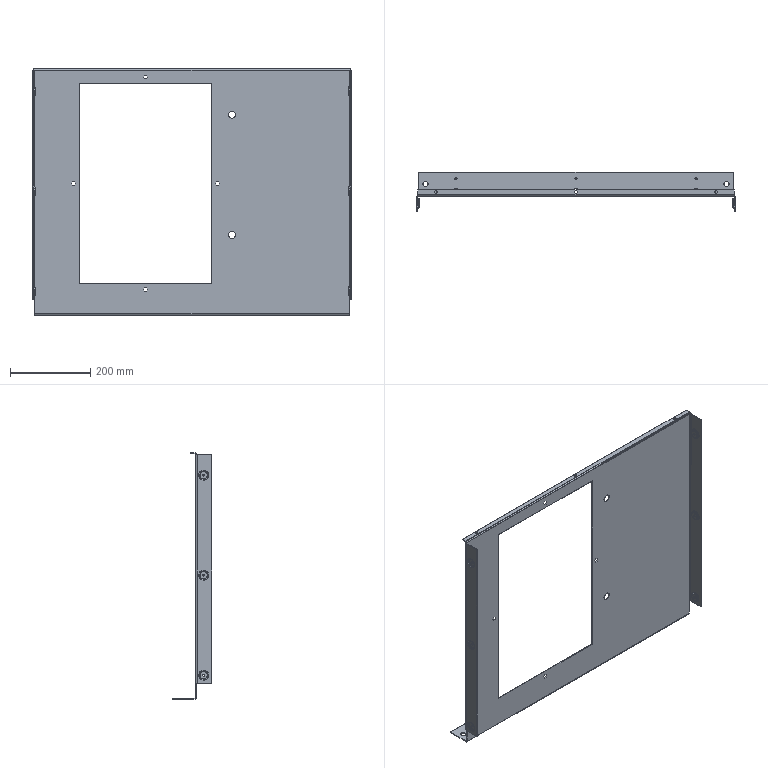Part | STEP file | 1 solid | 196 faces | box 795 x 98 x 616 mm | volume 839757 mm3 | plane 78 | cylinder 70 | torus 48 | commonest cylinder face diameters 4.7 x12 20 x12 24 x12 7 x10 13 x10 5.3 x6